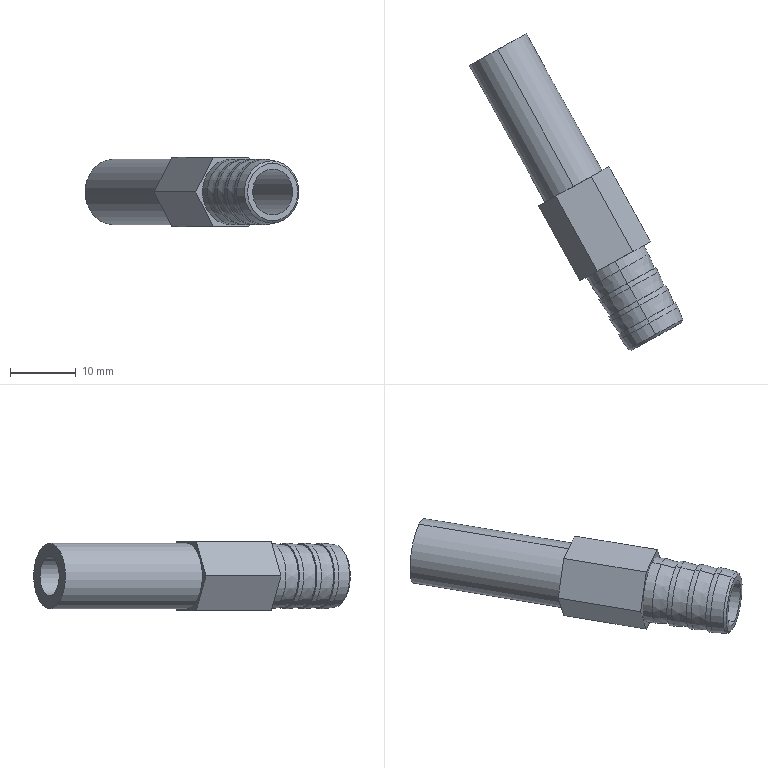Part | SolidWorks | features BaseBody 1 | 1 solid | 38 faces | box 32.611 x 48.276 x 10.659 mm | volume 2597 mm3 | cylinder 14 | plane 14 | cone 10 | commonest cylinder face diameters 10 x10 6 x2 7 x2
STEP:
#1=CARTESIAN_POINT('',(2.423,-77.341,-243.124));
#2=VERTEX_POINT('',#1);
#3=CARTESIAN_POINT('',(2.423,-77.341,-251.876));
#4=VERTEX_POINT('',#3);
#5=CARTESIAN_POINT('',(2.423,-77.341,-247.5));
#6=DIRECTION('',(-0.4848,0.8746,0.));
#7=DIRECTION('',(0.,0.,-1.));
#8=AXIS2_PLACEMENT_3D('',#5,#6,#7);
#9=CIRCLE('',#8,4.376);
#10=EDGE_CURVE('',#2,#4,#9,.T.);
#11=ORIENTED_EDGE('',*,*,#10,.T.);
#12=CARTESIAN_POINT('',(2.259,-77.045,-252.258));
#13=VERTEX_POINT('',#12);
#14=CARTESIAN_POINT('',(2.259,-77.045,-252.258));
#15=DIRECTION('',(-0.3212,0.5795,-0.749));
#16=VECTOR('',#15,1000.);
#17=LINE('',#14,#16);
#18=EDGE_CURVE('',#4,#13,#17,.T.);
#19=ORIENTED_EDGE('',*,*,#18,.T.);
#20=CARTESIAN_POINT('',(2.259,-77.045,-242.742));
#21=VERTEX_POINT('',#20);
#22=CARTESIAN_POINT('',(2.259,-77.045,-247.5));
#23=DIRECTION('',(0.4848,-0.8746,0.));
#24=DIRECTION('',(0.,0.,-1.));
#25=AXIS2_PLACEMENT_3D('',#22,#23,#24);
#26=CIRCLE('',#25,4.758);
#27=EDGE_CURVE('',#13,#21,#26,.T.);
#28=ORIENTED_EDGE('',*,*,#27,.T.);
#29=CARTESIAN_POINT('',(2.259,-77.045,-242.742));
#30=DIRECTION('',(-0.3212,0.5795,0.749));
#31=VECTOR('',#30,1000.);
#32=LINE('',#29,#31);
#33=EDGE_CURVE('',#2,#21,#32,.T.);
#34=ORIENTED_EDGE('',*,*,#33,.F.);
#35=EDGE_LOOP('',(#11,#19,#28,#34));
#36=FACE_OUTER_BOUND('',#35,.T.);
#37=CARTESIAN_POINT('',(2.259,-77.045,-247.5));
#38=DIRECTION('',(-0.4848,0.8746,0.));
#39=DIRECTION('',(0.,0.,1.));
#40=AXIS2_PLACEMENT_3D('',#37,#38,#39);
#41=CONICAL_SURFACE('',#40,4.758,0.8465);
#42=ADVANCED_FACE('',(#36),#41,.T.);
#43=CARTESIAN_POINT('',(-2.052,-69.267,-252.217));
#44=VERTEX_POINT('',#43);
#45=CARTESIAN_POINT('',(-2.052,-69.267,-242.783));
#46=VERTEX_POINT('',#45);
#47=CARTESIAN_POINT('',(-2.052,-69.267,-247.5));
#48=DIRECTION('',(0.4848,-0.8746,0.));
#49=DIRECTION('',(0.,0.,1.));
#50=AXIS2_PLACEMENT_3D('',#47,#48,#49);
#51=CIRCLE('',#50,4.717);
#52=EDGE_CURVE('',#44,#46,#51,.T.);
#53=ORIENTED_EDGE('',*,*,#52,.F.);
#54=CARTESIAN_POINT('',(-3.171,-67.249,-252.5));
#55=VERTEX_POINT('',#54);
#56=CARTESIAN_POINT('',(-3.171,-67.249,-252.5));
#57=DIRECTION('',(-0.4812,0.8681,-0.1219));
#58=VECTOR('',#57,1000.);
#59=LINE('',#56,#58);
#60=EDGE_CURVE('',#44,#55,#59,.T.);
#61=ORIENTED_EDGE('',*,*,#60,.T.);
#62=CARTESIAN_POINT('',(-3.171,-67.249,-242.5));
#63=VERTEX_POINT('',#62);
#64=CARTESIAN_POINT('',(-3.171,-67.249,-247.5));
#65=DIRECTION('',(0.4848,-0.8746,0.));
#66=DIRECTION('',(0.,0.,1.));
#67=AXIS2_PLACEMENT_3D('',#64,#65,#66);
#68=CIRCLE('',#67,5.);
#69=EDGE_CURVE('',#55,#63,#68,.T.);
#70=ORIENTED_EDGE('',*,*,#69,.T.);
#71=CARTESIAN_POINT('',(-3.171,-67.249,-242.5));
#72=DIRECTION('',(-0.4812,0.8681,0.1219));
#73=VECTOR('',#72,1000.);
#74=LINE('',#71,#73);
#75=EDGE_CURVE('',#46,#63,#74,.T.);
#76=ORIENTED_EDGE('',*,*,#75,.F.);
#77=EDGE_LOOP('',(#53,#61,#70,#76));
#78=FACE_OUTER_BOUND('',#77,.T.);
#79=CARTESIAN_POINT('',(-3.171,-67.249,-247.5));
#80=DIRECTION('',(-0.4848,0.8746,0.));
#81=DIRECTION('',(0.,0.,1.));
#82=AXIS2_PLACEMENT_3D('',#79,#80,#81);
#83=CONICAL_SURFACE('',#82,5.,0.1222);
#84=ADVANCED_FACE('',(#78),#83,.T.);
#85=CARTESIAN_POINT('',(-0.5605,-71.959,-252.217));
#86=VERTEX_POINT('',#85);
#87=CARTESIAN_POINT('',(-0.5605,-71.959,-242.783));
#88=VERTEX_POINT('',#87);
#89=CARTESIAN_POINT('',(-0.5605,-71.959,-247.5));
#90=DIRECTION('',(0.4848,-0.8746,0.));
#91=DIRECTION('',(0.,0.,1.));
#92=AXIS2_PLACEMENT_3D('',#89,#90,#91);
#93=CIRCLE('',#92,4.717);
#94=EDGE_CURVE('',#86,#88,#93,.T.);
#95=ORIENTED_EDGE('',*,*,#94,.F.);
#96=CARTESIAN_POINT('',(-1.679,-69.94,-252.5));
#97=VERTEX_POINT('',#96);
#98=CARTESIAN_POINT('',(-1.679,-69.94,-252.5));
#99=DIRECTION('',(-0.4812,0.8681,-0.1219));
#100=VECTOR('',#99,1000.);
#101=LINE('',#98,#100);
#102=EDGE_CURVE('',#86,#97,#101,.T.);
#103=ORIENTED_EDGE('',*,*,#102,.T.);
#104=CARTESIAN_POINT('',(-1.679,-69.94,-242.5));
#105=VERTEX_POINT('',#104);
#106=CARTESIAN_POINT('',(-1.679,-69.94,-247.5));
#107=DIRECTION('',(0.4848,-0.8746,0.));
#108=DIRECTION('',(0.,0.,1.));
#109=AXIS2_PLACEMENT_3D('',#106,#107,#108);
#110=CIRCLE('',#109,5.);
#111=EDGE_CURVE('',#97,#105,#110,.T.);
#112=ORIENTED_EDGE('',*,*,#111,.T.);
#113=CARTESIAN_POINT('',(-1.679,-69.94,-242.5));
#114=DIRECTION('',(-0.4812,0.8681,0.1219));
#115=VECTOR('',#114,1000.);
#116=LINE('',#113,#115);
#117=EDGE_CURVE('',#88,#105,#116,.T.);
#118=ORIENTED_EDGE('',*,*,#117,.F.);
#119=EDGE_LOOP('',(#95,#103,#112,#118));
#120=FACE_OUTER_BOUND('',#119,.T.);
#121=CARTESIAN_POINT('',(-1.679,-69.94,-247.5));
#122=DIRECTION('',(-0.4848,0.8746,0.));
#123=DIRECTION('',(0.,0.,1.));
#124=AXIS2_PLACEMENT_3D('',#121,#122,#123);
#125=CONICAL_SURFACE('',#124,5.,0.1222);
#126=ADVANCED_FACE('',(#120),#125,.T.);
#127=CARTESIAN_POINT('',(0.9313,-74.65,-252.217));
#128=VERTEX_POINT('',#127);
#129=CARTESIAN_POINT('',(0.9313,-74.65,-242.783));
#130=VERTEX_POINT('',#129);
#131=CARTESIAN_POINT('',(0.9313,-74.65,-247.5));
#132=DIRECTION('',(0.4848,-0.8746,0.));
#133=DIRECTION('',(0.,0.,1.));
#134=AXIS2_PLACEMENT_3D('',#131,#132,#133);
#135=CIRCLE('',#134,4.717);
#136=EDGE_CURVE('',#128,#130,#135,.T.);
#137=ORIENTED_EDGE('',*,*,#136,.F.);
#138=CARTESIAN_POINT('',(-0.1875,-72.631,-252.5));
#139=VERTEX_POINT('',#138);
#140=CARTESIAN_POINT('',(-0.1875,-72.631,-252.5));
#141=DIRECTION('',(-0.4812,0.8681,-0.1219));
#142=VECTOR('',#141,1000.);
#143=LINE('',#140,#142);
#144=EDGE_CURVE('',#128,#139,#143,.T.);
#145=ORIENTED_EDGE('',*,*,#144,.T.);
#146=CARTESIAN_POINT('',(-0.1875,-72.631,-242.5));
#147=VERTEX_POINT('',#146);
#148=CARTESIAN_POINT('',(-0.1875,-72.631,-247.5));
#149=DIRECTION('',(0.4848,-0.8746,0.));
#150=DIRECTION('',(0.,0.,1.));
#151=AXIS2_PLACEMENT_3D('',#148,#149,#150);
#152=CIRCLE('',#151,5.);
#153=EDGE_CURVE('',#139,#147,#152,.T.);
#154=ORIENTED_EDGE('',*,*,#153,.T.);
#155=CARTESIAN_POINT('',(-0.1875,-72.631,-242.5));
#156=DIRECTION('',(-0.4812,0.8681,0.1219));
#157=VECTOR('',#156,1000.);
#158=LINE('',#155,#157);
#159=EDGE_CURVE('',#130,#147,#158,.T.);
#160=ORIENTED_EDGE('',*,*,#159,.F.);
#161=EDGE_LOOP('',(#137,#145,#154,#160));
#162=FACE_OUTER_BOUND('',#161,.T.);
#163=CARTESIAN_POINT('',(-0.1875,-72.631,-247.5));
#164=DIRECTION('',(-0.4848,0.8746,0.));
#165=DIRECTION('',(0.,0.,1.));
#166=AXIS2_PLACEMENT_3D('',#163,#164,#165);
#167=CONICAL_SURFACE('',#166,5.,0.1222);
#168=ADVANCED_FACE('',(#162),#167,.T.);
#169=ORIENTED_EDGE('',*,*,#27,.F.);
#170=CARTESIAN_POINT('',(1.304,-75.322,-252.5));
#171=VERTEX_POINT('',#170);
#172=CARTESIAN_POINT('',(1.304,-75.322,-252.5));
#173=DIRECTION('',(-0.4812,0.8681,-0.1219));
#174=VECTOR('',#173,1000.);
#175=LINE('',#172,#174);
#176=EDGE_CURVE('',#13,#171,#175,.T.);
#177=ORIENTED_EDGE('',*,*,#176,.T.);
#178=CARTESIAN_POINT('',(1.304,-75.322,-242.5));
#179=VERTEX_POINT('',#178);
#180=CARTESIAN_POINT('',(1.304,-75.322,-247.5));
#181=DIRECTION('',(0.4848,-0.8746,0.));
#182=DIRECTION('',(0.,0.,1.));
#183=AXIS2_PLACEMENT_3D('',#180,#181,#182);
#184=CIRCLE('',#183,5.);
#185=EDGE_CURVE('',#171,#179,#184,.T.);
#186=ORIENTED_EDGE('',*,*,#185,.T.);
#187=CARTESIAN_POINT('',(1.304,-75.322,-242.5));
#188=DIRECTION('',(-0.4812,0.8681,0.1219));
#189=VECTOR('',#188,1000.);
#190=LINE('',#187,#189);
#191=EDGE_CURVE('',#21,#179,#190,.T.);
#192=ORIENTED_EDGE('',*,*,#191,.F.);
#193=EDGE_LOOP('',(#169,#177,#186,#192));
#194=FACE_OUTER_BOUND('',#193,.T.);
#195=CARTESIAN_POINT('',(1.304,-75.322,-247.5));
#196=DIRECTION('',(-0.4848,0.8746,0.));
#197=DIRECTION('',(0.,0.,1.));
#198=AXIS2_PLACEMENT_3D('',#195,#196,#197);
#199=CONICAL_SURFACE('',#198,5.,0.1222);
#200=ADVANCED_FACE('',(#194),#199,.T.);
#201=ORIENTED_EDGE('',*,*,#185,.F.);
#202=CARTESIAN_POINT('',(0.9313,-74.65,-252.5));
#203=VERTEX_POINT('',#202);
#204=CARTESIAN_POINT('',(2.423,-77.341,-252.5));
#205=DIRECTION('',(-0.4848,0.8746,0.));
#206=VECTOR('',#205,1000.);
#207=LINE('',#204,#206);
#208=EDGE_CURVE('',#171,#203,#207,.T.);
#209=ORIENTED_EDGE('',*,*,#208,.T.);
#210=CARTESIAN_POINT('',(0.9313,-74.65,-242.5));
#211=VERTEX_POINT('',#210);
#212=CARTESIAN_POINT('',(0.9313,-74.65,-247.5));
#213=DIRECTION('',(0.4848,-0.8746,0.));
#214=DIRECTION('',(0.,0.,1.));
#215=AXIS2_PLACEMENT_3D('',#212,#213,#214);
#216=CIRCLE('',#215,5.);
#217=EDGE_CURVE('',#203,#211,#216,.T.);
#218=ORIENTED_EDGE('',*,*,#217,.T.);
#219=CARTESIAN_POINT('',(2.423,-77.341,-242.5));
#220=DIRECTION('',(-0.4848,0.8746,0.));
#221=VECTOR('',#220,1000.);
#222=LINE('',#219,#221);
#223=EDGE_CURVE('',#179,#211,#222,.T.);
#224=ORIENTED_EDGE('',*,*,#223,.F.);
#225=EDGE_LOOP('',(#201,#209,#218,#224));
#226=FACE_OUTER_BOUND('',#225,.T.);
#227=CARTESIAN_POINT('',(2.423,-77.341,-247.5));
#228=DIRECTION('',(-0.4848,0.8746,0.));
#229=DIRECTION('',(0.,0.,1.));
#230=AXIS2_PLACEMENT_3D('',#227,#228,#229);
#231=CYLINDRICAL_SURFACE('',#230,5.);
#232=ADVANCED_FACE('',(#226),#231,.T.);
#233=ORIENTED_EDGE('',*,*,#153,.F.);
#234=CARTESIAN_POINT('',(-0.5605,-71.959,-252.5));
#235=VERTEX_POINT('',#234);
#236=CARTESIAN_POINT('',(2.423,-77.341,-252.5));
#237=DIRECTION('',(-0.4848,0.8746,0.));
#238=VECTOR('',#237,1000.);
#239=LINE('',#236,#238);
#240=EDGE_CURVE('',#139,#235,#239,.T.);
#241=ORIENTED_EDGE('',*,*,#240,.T.);
#242=CARTESIAN_POINT('',(-0.5605,-71.959,-242.5));
#243=VERTEX_POINT('',#242);
#244=CARTESIAN_POINT('',(-0.5605,-71.959,-247.5));
#245=DIRECTION('',(0.4848,-0.8746,0.));
#246=DIRECTION('',(0.,0.,1.));
#247=AXIS2_PLACEMENT_3D('',#244,#245,#246);
#248=CIRCLE('',#247,5.);
#249=EDGE_CURVE('',#235,#243,#248,.T.);
#250=ORIENTED_EDGE('',*,*,#249,.T.);
#251=CARTESIAN_POINT('',(2.423,-77.341,-242.5));
#252=DIRECTION('',(-0.4848,0.8746,0.));
#253=VECTOR('',#252,1000.);
#254=LINE('',#251,#253);
#255=EDGE_CURVE('',#147,#243,#254,.T.);
#256=ORIENTED_EDGE('',*,*,#255,.F.);
#257=EDGE_LOOP('',(#233,#241,#250,#256));
#258=FACE_OUTER_BOUND('',#257,.T.);
#259=CARTESIAN_POINT('',(2.423,-77.341,-247.5));
#260=DIRECTION('',(-0.4848,0.8746,0.));
#261=DIRECTION('',(0.,0.,1.));
#262=AXIS2_PLACEMENT_3D('',#259,#260,#261);
#263=CYLINDRICAL_SURFACE('',#262,5.);
#264=ADVANCED_FACE('',(#258),#263,.T.);
#265=ORIENTED_EDGE('',*,*,#111,.F.);
#266=CARTESIAN_POINT('',(-2.052,-69.267,-252.5));
#267=VERTEX_POINT('',#266);
#268=CARTESIAN_POINT('',(2.423,-77.341,-252.5));
#269=DIRECTION('',(-0.4848,0.8746,0.));
#270=VECTOR('',#269,1000.);
#271=LINE('',#268,#270);
#272=EDGE_CURVE('',#97,#267,#271,.T.);
#273=ORIENTED_EDGE('',*,*,#272,.T.);
#274=CARTESIAN_POINT('',(-2.052,-69.267,-242.5));
#275=VERTEX_POINT('',#274);
#276=CARTESIAN_POINT('',(-2.052,-69.267,-247.5));
#277=DIRECTION('',(0.4848,-0.8746,0.));
#278=DIRECTION('',(0.,0.,1.));
#279=AXIS2_PLACEMENT_3D('',#276,#277,#278);
#280=CIRCLE('',#279,5.);
#281=EDGE_CURVE('',#267,#275,#280,.T.);
#282=ORIENTED_EDGE('',*,*,#281,.T.);
#283=CARTESIAN_POINT('',(2.423,-77.341,-242.5));
#284=DIRECTION('',(-0.4848,0.8746,0.));
#285=VECTOR('',#284,1000.);
#286=LINE('',#283,#285);
#287=EDGE_CURVE('',#105,#275,#286,.T.);
#288=ORIENTED_EDGE('',*,*,#287,.F.);
#289=EDGE_LOOP('',(#265,#273,#282,#288));
#290=FACE_OUTER_BOUND('',#289,.T.);
#291=CARTESIAN_POINT('',(2.423,-77.341,-247.5));
#292=DIRECTION('',(-0.4848,0.8746,0.));
#293=DIRECTION('',(0.,0.,1.));
#294=AXIS2_PLACEMENT_3D('',#291,#292,#293);
#295=CYLINDRICAL_SURFACE('',#294,5.);
#296=ADVANCED_FACE('',(#290),#295,.T.);
#297=ORIENTED_EDGE('',*,*,#69,.F.);
#298=CARTESIAN_POINT('',(-3.917,-65.903,-252.5));
#299=VERTEX_POINT('',#298);
#300=CARTESIAN_POINT('',(-3.171,-67.249,-252.5));
#301=DIRECTION('',(-0.4848,0.8746,0.));
#302=VECTOR('',#301,1000.);
#303=LINE('',#300,#302);
#304=EDGE_CURVE('',#55,#299,#303,.T.);
#305=ORIENTED_EDGE('',*,*,#304,.T.);
#306=CARTESIAN_POINT('',(-3.917,-65.903,-242.5));
#307=VERTEX_POINT('',#306);
#308=CARTESIAN_POINT('',(-3.917,-65.903,-247.5));
#309=DIRECTION('',(0.4848,-0.8746,0.));
#310=DIRECTION('',(0.,0.,-1.));
#311=AXIS2_PLACEMENT_3D('',#308,#309,#310);
#312=CIRCLE('',#311,5.);
#313=EDGE_CURVE('',#299,#307,#312,.T.);
#314=ORIENTED_EDGE('',*,*,#313,.T.);
#315=CARTESIAN_POINT('',(-3.171,-67.249,-242.5));
#316=DIRECTION('',(-0.4848,0.8746,0.));
#317=VECTOR('',#316,1000.);
#318=LINE('',#315,#317);
#319=EDGE_CURVE('',#63,#307,#318,.T.);
#320=ORIENTED_EDGE('',*,*,#319,.F.);
#321=EDGE_LOOP('',(#297,#305,#314,#320));
#322=FACE_OUTER_BOUND('',#321,.T.);
#323=CARTESIAN_POINT('',(-3.171,-67.249,-247.5));
#324=DIRECTION('',(-0.4848,0.8746,0.));
#325=DIRECTION('',(0.,0.,1.));
#326=AXIS2_PLACEMENT_3D('',#323,#324,#325);
#327=CYLINDRICAL_SURFACE('',#326,5.);
#328=ADVANCED_FACE('',(#322),#327,.T.);
#329=CARTESIAN_POINT('',(-3.917,-65.903,-244.));
#330=VERTEX_POINT('',#329);
#331=CARTESIAN_POINT('',(-3.917,-65.903,-251.));
#332=VERTEX_POINT('',#331);
#333=CARTESIAN_POINT('',(-3.917,-65.903,-247.5));
#334=DIRECTION('',(0.4848,-0.8746,0.));
#335=DIRECTION('',(0.,0.,-1.));
#336=AXIS2_PLACEMENT_3D('',#333,#334,#335);
#337=CIRCLE('',#336,3.5);
#338=EDGE_CURVE('',#330,#332,#337,.T.);
#339=ORIENTED_EDGE('',*,*,#338,.F.);
#340=CARTESIAN_POINT('',(2.423,-77.341,-244.));
#341=VERTEX_POINT('',#340);
#342=CARTESIAN_POINT('',(-21.818,-33.61,-244.));
#343=DIRECTION('',(0.4848,-0.8746,0.));
#344=VECTOR('',#343,1000.);
#345=LINE('',#342,#344);
#346=EDGE_CURVE('',#330,#341,#345,.T.);
#347=ORIENTED_EDGE('',*,*,#346,.T.);
#348=CARTESIAN_POINT('',(2.423,-77.341,-251.));
#349=VERTEX_POINT('',#348);
#350=CARTESIAN_POINT('',(2.423,-77.341,-247.5));
#351=DIRECTION('',(-0.4848,0.8746,0.));
#352=DIRECTION('',(-0.586,-0.3248,0.7423));
#353=AXIS2_PLACEMENT_3D('',#350,#351,#352);
#354=CIRCLE('',#353,3.5);
#355=EDGE_CURVE('',#349,#341,#354,.T.);
#356=ORIENTED_EDGE('',*,*,#355,.F.);
#357=CARTESIAN_POINT('',(-21.818,-33.61,-251.));
#358=DIRECTION('',(0.4848,-0.8746,0.));
#359=VECTOR('',#358,1000.);
#360=LINE('',#357,#359);
#361=EDGE_CURVE('',#332,#349,#360,.T.);
#362=ORIENTED_EDGE('',*,*,#361,.F.);
#363=EDGE_LOOP('',(#339,#347,#356,#362));
#364=FACE_OUTER_BOUND('',#363,.T.);
#365=CARTESIAN_POINT('',(-21.818,-33.61,-247.5));
#366=DIRECTION('',(0.4848,-0.8746,0.));
#367=DIRECTION('',(0.,0.,-1.));
#368=AXIS2_PLACEMENT_3D('',#365,#366,#367);
#369=CYLINDRICAL_SURFACE('',#368,3.5);
#370=ADVANCED_FACE('',(#364),#369,.F.);
#371=CARTESIAN_POINT('',(-10.257,-54.466,-252.5));
#372=VERTEX_POINT('',#371);
#373=CARTESIAN_POINT('',(-10.257,-54.466,-242.5));
#374=VERTEX_POINT('',#373);
#375=CARTESIAN_POINT('',(-10.257,-54.466,-247.5));
#376=DIRECTION('',(0.4848,-0.8746,0.));
#377=DIRECTION('',(0.,0.,-1.));
#378=AXIS2_PLACEMENT_3D('',#375,#376,#377);
#379=CIRCLE('',#378,5.);
#380=EDGE_CURVE('',#372,#374,#379,.T.);
#381=ORIENTED_EDGE('',*,*,#380,.F.);
#382=CARTESIAN_POINT('',(-21.817,-33.611,-252.5));
#383=VERTEX_POINT('',#382);
#384=CARTESIAN_POINT('',(-60.602,36.359,-252.5));
#385=DIRECTION('',(-0.4848,0.8746,0.));
#386=VECTOR('',#385,1000.);
#387=LINE('',#384,#386);
#388=EDGE_CURVE('',#372,#383,#387,.T.);
#389=ORIENTED_EDGE('',*,*,#388,.T.);
#390=CARTESIAN_POINT('',(-21.817,-33.611,-242.5));
#391=VERTEX_POINT('',#390);
#392=CARTESIAN_POINT('',(-21.817,-33.611,-247.5));
#393=DIRECTION('',(0.4848,-0.8746,0.));
#394=DIRECTION('',(0.,0.,1.));
#395=AXIS2_PLACEMENT_3D('',#392,#393,#394);
#396=CIRCLE('',#395,5.);
#397=EDGE_CURVE('',#383,#391,#396,.T.);
#398=ORIENTED_EDGE('',*,*,#397,.T.);
#399=CARTESIAN_POINT('',(-60.602,36.359,-242.5));
#400=DIRECTION('',(-0.4848,0.8746,0.));
#401=VECTOR('',#400,1000.);
#402=LINE('',#399,#401);
#403=EDGE_CURVE('',#374,#391,#402,.T.);
#404=ORIENTED_EDGE('',*,*,#403,.F.);
#405=EDGE_LOOP('',(#381,#389,#398,#404));
#406=FACE_OUTER_BOUND('',#405,.T.);
#407=CARTESIAN_POINT('',(-60.602,36.359,-247.5));
#408=DIRECTION('',(-0.4848,0.8746,0.));
#409=DIRECTION('',(0.,0.,1.));
#410=AXIS2_PLACEMENT_3D('',#407,#408,#409);
#411=CYLINDRICAL_SURFACE('',#410,5.);
#412=ADVANCED_FACE('',(#406),#411,.T.);
#413=CARTESIAN_POINT('',(-3.917,-65.903,-244.5));
#414=VERTEX_POINT('',#413);
#415=CARTESIAN_POINT('',(-3.917,-65.903,-250.5));
#416=VERTEX_POINT('',#415);
#417=CARTESIAN_POINT('',(-3.917,-65.903,-247.5));
#418=DIRECTION('',(0.4848,-0.8746,0.));
#419=DIRECTION('',(0.,0.,-1.));
#420=AXIS2_PLACEMENT_3D('',#417,#418,#419);
#421=CIRCLE('',#420,3.);
#422=EDGE_CURVE('',#414,#416,#421,.T.);
#423=ORIENTED_EDGE('',*,*,#422,.T.);
#424=CARTESIAN_POINT('',(-21.817,-33.611,-250.5));
#425=VERTEX_POINT('',#424);
#426=CARTESIAN_POINT('',(-5.818,-62.473,-250.5));
#427=DIRECTION('',(-0.4848,0.8746,0.));
#428=VECTOR('',#427,1000.);
#429=LINE('',#426,#428);
#430=EDGE_CURVE('',#416,#425,#429,.T.);
#431=ORIENTED_EDGE('',*,*,#430,.T.);
#432=CARTESIAN_POINT('',(-21.817,-33.611,-244.5));
#433=VERTEX_POINT('',#432);
#434=CARTESIAN_POINT('',(-21.817,-33.611,-247.5));
#435=DIRECTION('',(-0.4848,0.8746,0.));
#436=DIRECTION('',(0.,0.,1.));
#437=AXIS2_PLACEMENT_3D('',#434,#435,#436);
#438=CIRCLE('',#437,3.);
#439=EDGE_CURVE('',#425,#433,#438,.T.);
#440=ORIENTED_EDGE('',*,*,#439,.T.);
#441=CARTESIAN_POINT('',(-5.818,-62.473,-244.5));
#442=DIRECTION('',(-0.4848,0.8746,0.));
#443=VECTOR('',#442,1000.);
#444=LINE('',#441,#443);
#445=EDGE_CURVE('',#414,#433,#444,.T.);
#446=ORIENTED_EDGE('',*,*,#445,.F.);
#447=EDGE_LOOP('',(#423,#431,#440,#446));
#448=FACE_OUTER_BOUND('',#447,.T.);
#449=CARTESIAN_POINT('',(-5.818,-62.473,-247.5));
#450=DIRECTION('',(-0.4848,0.8746,0.));
#451=DIRECTION('',(0.,0.,1.));
#452=AXIS2_PLACEMENT_3D('',#449,#450,#451);
#453=CYLINDRICAL_SURFACE('',#452,3.);
#454=ADVANCED_FACE('',(#448),#453,.F.);
#455=ORIENTED_EDGE('',*,*,#430,.F.);
#456=CARTESIAN_POINT('',(-3.917,-65.903,-247.5));
#457=DIRECTION('',(0.4848,-0.8746,0.));
#458=DIRECTION('',(0.,0.,-1.));
#459=AXIS2_PLACEMENT_3D('',#456,#457,#458);
#460=CIRCLE('',#459,3.);
#461=EDGE_CURVE('',#416,#414,#460,.T.);
#462=ORIENTED_EDGE('',*,*,#461,.T.);
#463=ORIENTED_EDGE('',*,*,#445,.T.);
#464=CARTESIAN_POINT('',(-21.817,-33.611,-247.5));
#465=DIRECTION('',(-0.4848,0.8746,0.));
#466=DIRECTION('',(0.,0.,1.));
#467=AXIS2_PLACEMENT_3D('',#464,#465,#466);
#468=CIRCLE('',#467,3.);
#469=EDGE_CURVE('',#433,#425,#468,.T.);
#470=ORIENTED_EDGE('',*,*,#469,.T.);
#471=EDGE_LOOP('',(#455,#462,#463,#470));
#472=FACE_OUTER_BOUND('',#471,.T.);
#473=CARTESIAN_POINT('',(-5.818,-62.473,-247.5));
#474=DIRECTION('',(-0.4848,0.8746,0.));
#475=DIRECTION('',(0.,0.,1.));
#476=AXIS2_PLACEMENT_3D('',#473,#474,#475);
#477=CYLINDRICAL_SURFACE('',#476,3.);
#478=ADVANCED_FACE('',(#472),#477,.F.);
#479=ORIENTED_EDGE('',*,*,#388,.F.);
#480=CARTESIAN_POINT('',(-10.257,-54.466,-247.5));
#481=DIRECTION('',(0.4848,-0.8746,0.));
#482=DIRECTION('',(0.,0.,-1.));
#483=AXIS2_PLACEMENT_3D('',#480,#481,#482);
#484=CIRCLE('',#483,5.);
#485=EDGE_CURVE('',#374,#372,#484,.T.);
#486=ORIENTED_EDGE('',*,*,#485,.F.);
#487=ORIENTED_EDGE('',*,*,#403,.T.);
#488=CARTESIAN_POINT('',(-21.817,-33.611,-247.5));
#489=DIRECTION('',(0.4848,-0.8746,0.));
#490=DIRECTION('',(0.,0.,1.));
#491=AXIS2_PLACEMENT_3D('',#488,#489,#490);
#492=CIRCLE('',#491,5.);
#493=EDGE_CURVE('',#391,#383,#492,.T.);
#494=ORIENTED_EDGE('',*,*,#493,.T.);
#495=EDGE_LOOP('',(#479,#486,#487,#494));
#496=FACE_OUTER_BOUND('',#495,.T.);
#497=CARTESIAN_POINT('',(-60.602,36.359,-247.5));
#498=DIRECTION('',(-0.4848,0.8746,0.));
#499=DIRECTION('',(0.,0.,1.));
#500=AXIS2_PLACEMENT_3D('',#497,#498,#499);
#501=CYLINDRICAL_SURFACE('',#500,5.);
#502=ADVANCED_FACE('',(#496),#501,.T.);
#503=CARTESIAN_POINT('',(-3.917,-65.903,-247.5));
#504=DIRECTION('',(0.4848,-0.8746,0.));
#505=DIRECTION('',(0.,0.,-1.));
#506=AXIS2_PLACEMENT_3D('',#503,#504,#505);
#507=CIRCLE('',#506,3.5);
#508=EDGE_CURVE('',#332,#330,#507,.T.);
#509=ORIENTED_EDGE('',*,*,#508,.T.);
#510=ORIENTED_EDGE('',*,*,#338,.T.);
#511=EDGE_LOOP('',(#509,#510));
#512=FACE_OUTER_BOUND('',#511,.T.);
#513=ORIENTED_EDGE('',*,*,#422,.F.);
#514=ORIENTED_EDGE('',*,*,#461,.F.);
#515=EDGE_LOOP('',(#513,#514));
#516=FACE_BOUND('',#515,.T.);
#517=CARTESIAN_POINT('',(-3.917,-65.903,-247.5));
#518=DIRECTION('',(0.4848,-0.8746,0.));
#519=DIRECTION('',(0.,0.,1.));
#520=AXIS2_PLACEMENT_3D('',#517,#518,#519);
#521=PLANE('',#520);
#522=ADVANCED_FACE('',(#512,#516),#521,.T.);
#523=ORIENTED_EDGE('',*,*,#346,.F.);
#524=ORIENTED_EDGE('',*,*,#508,.F.);
#525=ORIENTED_EDGE('',*,*,#361,.T.);
#526=CARTESIAN_POINT('',(2.423,-77.341,-247.5));
#527=DIRECTION('',(-0.4848,0.8746,0.));
#528=DIRECTION('',(-0.586,-0.3248,0.7423));
#529=AXIS2_PLACEMENT_3D('',#526,#527,#528);
#530=CIRCLE('',#529,3.5);
#531=EDGE_CURVE('',#341,#349,#530,.T.);
#532=ORIENTED_EDGE('',*,*,#531,.F.);
#533=EDGE_LOOP('',(#523,#524,#525,#532));
#534=FACE_OUTER_BOUND('',#533,.T.);
#535=CARTESIAN_POINT('',(-21.818,-33.61,-247.5));
#536=DIRECTION('',(0.4848,-0.8746,0.));
#537=DIRECTION('',(0.,0.,-1.));
#538=AXIS2_PLACEMENT_3D('',#535,#536,#537);
#539=CYLINDRICAL_SURFACE('',#538,3.5);
#540=ADVANCED_FACE('',(#534),#539,.F.);
#541=CARTESIAN_POINT('',(-4.874,-51.483,-247.5));
#542=VERTEX_POINT('',#541);
#543=CARTESIAN_POINT('',(-7.566,-52.974,-242.171));
#544=VERTEX_POINT('',#543);
#545=CARTESIAN_POINT('',(-4.874,-51.483,-247.5));
#546=DIRECTION('',(-0.4373,-0.2424,0.866));
#547=VECTOR('',#546,1000.);
#548=LINE('',#545,#547);
#549=EDGE_CURVE('',#542,#544,#548,.T.);
#550=ORIENTED_EDGE('',*,*,#549,.F.);
#551=CARTESIAN_POINT('',(-7.566,-52.974,-252.829));
#552=VERTEX_POINT('',#551);
#553=CARTESIAN_POINT('',(-7.566,-52.974,-252.829));
#554=DIRECTION('',(0.4373,0.2424,0.866));
#555=VECTOR('',#554,1000.);
#556=LINE('',#553,#555);
#557=EDGE_CURVE('',#552,#542,#556,.T.);
#558=ORIENTED_EDGE('',*,*,#557,.F.);
#559=CARTESIAN_POINT('',(-12.948,-55.958,-252.829));
#560=VERTEX_POINT('',#559);
#561=CARTESIAN_POINT('',(-12.948,-55.958,-252.829));
#562=DIRECTION('',(0.8746,0.4848,0.));
#563=VECTOR('',#562,1000.);
#564=LINE('',#561,#563);
#565=EDGE_CURVE('',#560,#552,#564,.T.);
#566=ORIENTED_EDGE('',*,*,#565,.F.);
#567=CARTESIAN_POINT('',(-15.639,-57.45,-247.5));
#568=VERTEX_POINT('',#567);
#569=CARTESIAN_POINT('',(-15.639,-57.45,-247.5));
#570=DIRECTION('',(0.4373,0.2424,-0.866));
#571=VECTOR('',#570,1000.);
#572=LINE('',#569,#571);
#573=EDGE_CURVE('',#568,#560,#572,.T.);
#574=ORIENTED_EDGE('',*,*,#573,.F.);
#575=CARTESIAN_POINT('',(-12.948,-55.958,-242.171));
#576=VERTEX_POINT('',#575);
#577=CARTESIAN_POINT('',(-12.948,-55.958,-242.171));
#578=DIRECTION('',(-0.4373,-0.2424,-0.866));
#579=VECTOR('',#578,1000.);
#580=LINE('',#577,#579);
#581=EDGE_CURVE('',#576,#568,#580,.T.);
#582=ORIENTED_EDGE('',*,*,#581,.F.);
#583=CARTESIAN_POINT('',(-7.566,-52.974,-242.171));
#584=DIRECTION('',(-0.8746,-0.4848,0.));
#585=VECTOR('',#584,1000.);
#586=LINE('',#583,#585);
#587=EDGE_CURVE('',#544,#576,#586,.T.);
#588=ORIENTED_EDGE('',*,*,#587,.F.);
#589=EDGE_LOOP('',(#550,#558,#566,#574,#582,#588));
#590=FACE_OUTER_BOUND('',#589,.T.);
#591=ORIENTED_EDGE('',*,*,#485,.T.);
#592=ORIENTED_EDGE('',*,*,#380,.T.);
#593=EDGE_LOOP('',(#591,#592));
#594=FACE_BOUND('',#593,.T.);
#595=CARTESIAN_POINT('',(-10.257,-54.466,-247.5));
#596=DIRECTION('',(0.4848,-0.8746,0.));
#597=DIRECTION('',(0.,0.,1.));
#598=AXIS2_PLACEMENT_3D('',#595,#596,#597);
#599=PLANE('',#598);
#600=ADVANCED_FACE('',(#590,#594),#599,.F.);
#601=CARTESIAN_POINT('',(-1.226,-64.412,-252.829));
#602=VERTEX_POINT('',#601);
#603=CARTESIAN_POINT('',(1.465,-62.92,-247.5));
#604=VERTEX_POINT('',#603);
#605=CARTESIAN_POINT('',(-1.226,-64.412,-252.829));
#606=DIRECTION('',(0.4373,0.2424,0.866));
#607=VECTOR('',#606,1000.);
#608=LINE('',#605,#607);
#609=EDGE_CURVE('',#602,#604,#608,.T.);
#610=ORIENTED_EDGE('',*,*,#609,.F.);
#611=CARTESIAN_POINT('',(-9.803,-48.938,-252.829));
#612=DIRECTION('',(0.4848,-0.8746,0.));
#613=VECTOR('',#612,1000.);
#614=LINE('',#611,#613);
#615=EDGE_CURVE('',#552,#602,#614,.T.);
#616=ORIENTED_EDGE('',*,*,#615,.F.);
#617=ORIENTED_EDGE('',*,*,#557,.T.);
#618=CARTESIAN_POINT('',(-7.112,-47.446,-247.5));
#619=DIRECTION('',(0.4848,-0.8746,0.));
#620=VECTOR('',#619,1000.);
#621=LINE('',#618,#620);
#622=EDGE_CURVE('',#542,#604,#621,.T.);
#623=ORIENTED_EDGE('',*,*,#622,.T.);
#624=EDGE_LOOP('',(#610,#616,#617,#623));
#625=FACE_OUTER_BOUND('',#624,.T.);
#626=CARTESIAN_POINT('',(-9.803,-48.938,-252.829));
#627=DIRECTION('',(0.7574,0.4199,-0.5));
#628=DIRECTION('',(0.4373,0.2424,0.866));
#629=AXIS2_PLACEMENT_3D('',#626,#627,#628);
#630=PLANE('',#629);
#631=ADVANCED_FACE('',(#625),#630,.T.);
#632=CARTESIAN_POINT('',(-6.608,-67.395,-252.829));
#633=VERTEX_POINT('',#632);
#634=CARTESIAN_POINT('',(-6.608,-67.395,-252.829));
#635=DIRECTION('',(0.8746,0.4848,0.));
#636=VECTOR('',#635,1000.);
#637=LINE('',#634,#636);
#638=EDGE_CURVE('',#633,#602,#637,.T.);
#639=ORIENTED_EDGE('',*,*,#638,.F.);
#640=CARTESIAN_POINT('',(-15.185,-51.921,-252.829));
#641=DIRECTION('',(0.4848,-0.8746,0.));
#642=VECTOR('',#641,1000.);
#643=LINE('',#640,#642);
#644=EDGE_CURVE('',#560,#633,#643,.T.);
#645=ORIENTED_EDGE('',*,*,#644,.F.);
#646=ORIENTED_EDGE('',*,*,#565,.T.);
#647=ORIENTED_EDGE('',*,*,#615,.T.);
#648=EDGE_LOOP('',(#639,#645,#646,#647));
#649=FACE_OUTER_BOUND('',#648,.T.);
#650=CARTESIAN_POINT('',(-15.185,-51.921,-252.829));
#651=DIRECTION('',(0.,0.,-1.));
#652=DIRECTION('',(0.8746,0.4848,0.));
#653=AXIS2_PLACEMENT_3D('',#650,#651,#652);
#654=PLANE('',#653);
#655=ADVANCED_FACE('',(#649),#654,.T.);
#656=CARTESIAN_POINT('',(-9.299,-68.887,-247.5));
#657=VERTEX_POINT('',#656);
#658=CARTESIAN_POINT('',(-9.299,-68.887,-247.5));
#659=DIRECTION('',(0.4373,0.2424,-0.866));
#660=VECTOR('',#659,1000.);
#661=LINE('',#658,#660);
#662=EDGE_CURVE('',#657,#633,#661,.T.);
#663=ORIENTED_EDGE('',*,*,#662,.F.);
#664=CARTESIAN_POINT('',(-17.877,-53.413,-247.5));
#665=DIRECTION('',(0.4848,-0.8746,0.));
#666=VECTOR('',#665,1000.);
#667=LINE('',#664,#666);
#668=EDGE_CURVE('',#568,#657,#667,.T.);
#669=ORIENTED_EDGE('',*,*,#668,.F.);
#670=ORIENTED_EDGE('',*,*,#573,.T.);
#671=ORIENTED_EDGE('',*,*,#644,.T.);
#672=EDGE_LOOP('',(#663,#669,#670,#671));
#673=FACE_OUTER_BOUND('',#672,.T.);
#674=CARTESIAN_POINT('',(-17.877,-53.413,-247.5));
#675=DIRECTION('',(-0.7574,-0.4199,-0.5));
#676=DIRECTION('',(0.4373,0.2424,-0.866));
#677=AXIS2_PLACEMENT_3D('',#674,#675,#676);
#678=PLANE('',#677);
#679=ADVANCED_FACE('',(#673),#678,.T.);
#680=CARTESIAN_POINT('',(-6.608,-67.395,-242.171));
#681=VERTEX_POINT('',#680);
#682=CARTESIAN_POINT('',(-6.608,-67.395,-242.171));
#683=DIRECTION('',(-0.4373,-0.2424,-0.866));
#684=VECTOR('',#683,1000.);
#685=LINE('',#682,#684);
#686=EDGE_CURVE('',#681,#657,#685,.T.);
#687=ORIENTED_EDGE('',*,*,#686,.F.);
#688=CARTESIAN_POINT('',(-15.185,-51.921,-242.171));
#689=DIRECTION('',(0.4848,-0.8746,0.));
#690=VECTOR('',#689,1000.);
#691=LINE('',#688,#690);
#692=EDGE_CURVE('',#576,#681,#691,.T.);
#693=ORIENTED_EDGE('',*,*,#692,.F.);
#694=ORIENTED_EDGE('',*,*,#581,.T.);
#695=ORIENTED_EDGE('',*,*,#668,.T.);
#696=EDGE_LOOP('',(#687,#693,#694,#695));
#697=FACE_OUTER_BOUND('',#696,.T.);
#698=CARTESIAN_POINT('',(-15.185,-51.921,-242.171));
#699=DIRECTION('',(-0.7574,-0.4199,0.5));
#700=DIRECTION('',(-0.4373,-0.2424,-0.866));
#701=AXIS2_PLACEMENT_3D('',#698,#699,#700);
#702=PLANE('',#701);
#703=ADVANCED_FACE('',(#697),#702,.T.);
#704=CARTESIAN_POINT('',(-1.226,-64.412,-242.171));
#705=VERTEX_POINT('',#704);
#706=CARTESIAN_POINT('',(-1.226,-64.412,-242.171));
#707=DIRECTION('',(-0.8746,-0.4848,0.));
#708=VECTOR('',#707,1000.);
#709=LINE('',#706,#708);
#710=EDGE_CURVE('',#705,#681,#709,.T.);
#711=ORIENTED_EDGE('',*,*,#710,.F.);
#712=CARTESIAN_POINT('',(-9.803,-48.938,-242.171));
#713=DIRECTION('',(0.4848,-0.8746,0.));
#714=VECTOR('',#713,1000.);
#715=LINE('',#712,#714);
#716=EDGE_CURVE('',#544,#705,#715,.T.);
#717=ORIENTED_EDGE('',*,*,#716,.F.);
#718=ORIENTED_EDGE('',*,*,#587,.T.);
#719=ORIENTED_EDGE('',*,*,#692,.T.);
#720=EDGE_LOOP('',(#711,#717,#718,#719));
#721=FACE_OUTER_BOUND('',#720,.T.);
#722=CARTESIAN_POINT('',(-9.803,-48.938,-242.171));
#723=DIRECTION('',(0.,0.,1.));
#724=DIRECTION('',(-0.8746,-0.4848,0.));
#725=AXIS2_PLACEMENT_3D('',#722,#723,#724);
#726=PLANE('',#725);
#727=ADVANCED_FACE('',(#721),#726,.T.);
#728=ORIENTED_EDGE('',*,*,#622,.F.);
#729=ORIENTED_EDGE('',*,*,#549,.T.);
#730=ORIENTED_EDGE('',*,*,#716,.T.);
#731=CARTESIAN_POINT('',(1.465,-62.92,-247.5));
#732=DIRECTION('',(-0.4373,-0.2424,0.866));
#733=VECTOR('',#732,1000.);
#734=LINE('',#731,#733);
#735=EDGE_CURVE('',#604,#705,#734,.T.);
#736=ORIENTED_EDGE('',*,*,#735,.F.);
#737=EDGE_LOOP('',(#728,#729,#730,#736));
#738=FACE_OUTER_BOUND('',#737,.T.);
#739=CARTESIAN_POINT('',(-7.112,-47.446,-247.5));
#740=DIRECTION('',(0.7574,0.4199,0.5));
#741=DIRECTION('',(-0.4373,-0.2424,0.866));
#742=AXIS2_PLACEMENT_3D('',#739,#740,#741);
#743=PLANE('',#742);
#744=ADVANCED_FACE('',(#738),#743,.T.);
#745=ORIENTED_EDGE('',*,*,#304,.F.);
#746=CARTESIAN_POINT('',(-3.171,-67.249,-247.5));
#747=DIRECTION('',(0.4848,-0.8746,0.));
#748=DIRECTION('',(0.,0.,1.));
#749=AXIS2_PLACEMENT_3D('',#746,#747,#748);
#750=CIRCLE('',#749,5.);
#751=EDGE_CURVE('',#63,#55,#750,.T.);
#752=ORIENTED_EDGE('',*,*,#751,.F.);
#753=ORIENTED_EDGE('',*,*,#319,.T.);
#754=CARTESIAN_POINT('',(-3.917,-65.903,-247.5));
#755=DIRECTION('',(0.4848,-0.8746,0.));
#756=DIRECTION('',(0.,0.,-1.));
#757=AXIS2_PLACEMENT_3D('',#754,#755,#756);
#758=CIRCLE('',#757,5.);
#759=EDGE_CURVE('',#307,#299,#758,.T.);
#760=ORIENTED_EDGE('',*,*,#759,.T.);
#761=EDGE_LOOP('',(#745,#752,#753,#760));
#762=FACE_OUTER_BOUND('',#761,.T.);
#763=CARTESIAN_POINT('',(-3.171,-67.249,-247.5));
#764=DIRECTION('',(-0.4848,0.8746,0.));
#765=DIRECTION('',(0.,0.,1.));
#766=AXIS2_PLACEMENT_3D('',#763,#764,#765);
#767=CYLINDRICAL_SURFACE('',#766,5.);
#768=ADVANCED_FACE('',(#762),#767,.T.);
#769=ORIENTED_EDGE('',*,*,#272,.F.);
#770=CARTESIAN_POINT('',(-1.679,-69.94,-247.5));
#771=DIRECTION('',(0.4848,-0.8746,0.));
#772=DIRECTION('',(0.,0.,1.));
#773=AXIS2_PLACEMENT_3D('',#770,#771,#772);
#774=CIRCLE('',#773,5.);
#775=EDGE_CURVE('',#105,#97,#774,.T.);
#776=ORIENTED_EDGE('',*,*,#775,.F.);
#777=ORIENTED_EDGE('',*,*,#287,.T.);
#778=CARTESIAN_POINT('',(-2.052,-69.267,-247.5));
#779=DIRECTION('',(0.4848,-0.8746,0.));
#780=DIRECTION('',(0.,0.,1.));
#781=AXIS2_PLACEMENT_3D('',#778,#779,#780);
#782=CIRCLE('',#781,5.);
#783=EDGE_CURVE('',#275,#267,#782,.T.);
#784=ORIENTED_EDGE('',*,*,#783,.T.);
#785=EDGE_LOOP('',(#769,#776,#777,#784));
#786=FACE_OUTER_BOUND('',#785,.T.);
#787=CARTESIAN_POINT('',(2.423,-77.341,-247.5));
#788=DIRECTION('',(-0.4848,0.8746,0.));
#789=DIRECTION('',(0.,0.,1.));
#790=AXIS2_PLACEMENT_3D('',#787,#788,#789);
#791=CYLINDRICAL_SURFACE('',#790,5.);
#792=ADVANCED_FACE('',(#786),#791,.T.);
#793=ORIENTED_EDGE('',*,*,#240,.F.);
#794=CARTESIAN_POINT('',(-0.1875,-72.631,-247.5));
#795=DIRECTION('',(0.4848,-0.8746,0.));
#796=DIRECTION('',(0.,0.,1.));
#797=AXIS2_PLACEMENT_3D('',#794,#795,#796);
#798=CIRCLE('',#797,5.);
#799=EDGE_CURVE('',#147,#139,#798,.T.);
#800=ORIENTED_EDGE('',*,*,#799,.F.);
#801=ORIENTED_EDGE('',*,*,#255,.T.);
#802=CARTESIAN_POINT('',(-0.5605,-71.959,-247.5));
#803=DIRECTION('',(0.4848,-0.8746,0.));
#804=DIRECTION('',(0.,0.,1.));
#805=AXIS2_PLACEMENT_3D('',#802,#803,#804);
#806=CIRCLE('',#805,5.);
#807=EDGE_CURVE('',#243,#235,#806,.T.);
#808=ORIENTED_EDGE('',*,*,#807,.T.);
#809=EDGE_LOOP('',(#793,#800,#801,#808));
#810=FACE_OUTER_BOUND('',#809,.T.);
#811=CARTESIAN_POINT('',(2.423,-77.341,-247.5));
#812=DIRECTION('',(-0.4848,0.8746,0.));
#813=DIRECTION('',(0.,0.,1.));
#814=AXIS2_PLACEMENT_3D('',#811,#812,#813);
#815=CYLINDRICAL_SURFACE('',#814,5.);
#816=ADVANCED_FACE('',(#810),#815,.T.);
#817=ORIENTED_EDGE('',*,*,#208,.F.);
#818=CARTESIAN_POINT('',(1.304,-75.322,-247.5));
#819=DIRECTION('',(0.4848,-0.8746,0.));
#820=DIRECTION('',(0.,0.,1.));
#821=AXIS2_PLACEMENT_3D('',#818,#819,#820);
#822=CIRCLE('',#821,5.);
#823=EDGE_CURVE('',#179,#171,#822,.T.);
#824=ORIENTED_EDGE('',*,*,#823,.F.);
#825=ORIENTED_EDGE('',*,*,#223,.T.);
#826=CARTESIAN_POINT('',(0.9313,-74.65,-247.5));
#827=DIRECTION('',(0.4848,-0.8746,0.));
#828=DIRECTION('',(0.,0.,1.));
#829=AXIS2_PLACEMENT_3D('',#826,#827,#828);
#830=CIRCLE('',#829,5.);
#831=EDGE_CURVE('',#211,#203,#830,.T.);
#832=ORIENTED_EDGE('',*,*,#831,.T.);
#833=EDGE_LOOP('',(#817,#824,#825,#832));
#834=FACE_OUTER_BOUND('',#833,.T.);
#835=CARTESIAN_POINT('',(2.423,-77.341,-247.5));
#836=DIRECTION('',(-0.4848,0.8746,0.));
#837=DIRECTION('',(0.,0.,1.));
#838=AXIS2_PLACEMENT_3D('',#835,#836,#837);
#839=CYLINDRICAL_SURFACE('',#838,5.);
#840=ADVANCED_FACE('',(#834),#839,.T.);
#841=ORIENTED_EDGE('',*,*,#355,.T.);
#842=ORIENTED_EDGE('',*,*,#531,.T.);
#843=EDGE_LOOP('',(#841,#842));
#844=FACE_BOUND('',#843,.T.);
#845=ORIENTED_EDGE('',*,*,#10,.F.);
#846=CARTESIAN_POINT('',(2.423,-77.341,-247.5));
#847=DIRECTION('',(-0.4848,0.8746,0.));
#848=DIRECTION('',(0.,0.,-1.));
#849=AXIS2_PLACEMENT_3D('',#846,#847,#848);
#850=CIRCLE('',#849,4.376);
#851=EDGE_CURVE('',#4,#2,#850,.T.);
#852=ORIENTED_EDGE('',*,*,#851,.F.);
#853=EDGE_LOOP('',(#845,#852));
#854=FACE_OUTER_BOUND('',#853,.T.);
#855=CARTESIAN_POINT('',(2.423,-77.341,-247.5));
#856=DIRECTION('',(0.4848,-0.8746,0.));
#857=DIRECTION('',(0.,0.,-1.));
#858=AXIS2_PLACEMENT_3D('',#855,#856,#857);
#859=PLANE('',#858);
#860=ADVANCED_FACE('',(#844,#854),#859,.T.);
#861=ORIENTED_EDGE('',*,*,#176,.F.);
#862=CARTESIAN_POINT('',(2.259,-77.045,-247.5));
#863=DIRECTION('',(0.4848,-0.8746,0.));
#864=DIRECTION('',(0.,0.,-1.));
#865=AXIS2_PLACEMENT_3D('',#862,#863,#864);
#866=CIRCLE('',#865,4.758);
#867=EDGE_CURVE('',#21,#13,#866,.T.);
#868=ORIENTED_EDGE('',*,*,#867,.F.);
#869=ORIENTED_EDGE('',*,*,#191,.T.);
#870=ORIENTED_EDGE('',*,*,#823,.T.);
#871=EDGE_LOOP('',(#861,#868,#869,#870));
#872=FACE_OUTER_BOUND('',#871,.T.);
#873=CARTESIAN_POINT('',(1.304,-75.322,-247.5));
#874=DIRECTION('',(-0.4848,0.8746,0.));
#875=DIRECTION('',(0.,0.,1.));
#876=AXIS2_PLACEMENT_3D('',#873,#874,#875);
#877=CONICAL_SURFACE('',#876,5.,0.1222);
#878=ADVANCED_FACE('',(#872),#877,.T.);
#879=CARTESIAN_POINT('',(0.9313,-74.65,-247.5));
#880=DIRECTION('',(0.4848,-0.8746,0.));
#881=DIRECTION('',(0.,0.,1.));
#882=AXIS2_PLACEMENT_3D('',#879,#880,#881);
#883=CIRCLE('',#882,4.717);
#884=EDGE_CURVE('',#130,#128,#883,.T.);
#885=ORIENTED_EDGE('',*,*,#884,.T.);
#886=ORIENTED_EDGE('',*,*,#136,.T.);
#887=EDGE_LOOP('',(#885,#886));
#888=FACE_BOUND('',#887,.T.);
#889=ORIENTED_EDGE('',*,*,#831,.F.);
#890=ORIENTED_EDGE('',*,*,#217,.F.);
#891=EDGE_LOOP('',(#889,#890));
#892=FACE_OUTER_BOUND('',#891,.T.);
#893=CARTESIAN_POINT('',(0.9313,-74.65,-252.217));
#894=DIRECTION('',(-0.4848,0.8746,0.));
#895=DIRECTION('',(0.,0.,1.));
#896=AXIS2_PLACEMENT_3D('',#893,#894,#895);
#897=PLANE('',#896);
#898=ADVANCED_FACE('',(#888,#892),#897,.T.);
#899=ORIENTED_EDGE('',*,*,#144,.F.);
#900=ORIENTED_EDGE('',*,*,#884,.F.);
#901=ORIENTED_EDGE('',*,*,#159,.T.);
#902=ORIENTED_EDGE('',*,*,#799,.T.);
#903=EDGE_LOOP('',(#899,#900,#901,#902));
#904=FACE_OUTER_BOUND('',#903,.T.);
#905=CARTESIAN_POINT('',(-0.1875,-72.631,-247.5));
#906=DIRECTION('',(-0.4848,0.8746,0.));
#907=DIRECTION('',(0.,0.,1.));
#908=AXIS2_PLACEMENT_3D('',#905,#906,#907);
#909=CONICAL_SURFACE('',#908,5.,0.1222);
#910=ADVANCED_FACE('',(#904),#909,.T.);
#911=CARTESIAN_POINT('',(-0.5605,-71.959,-247.5));
#912=DIRECTION('',(0.4848,-0.8746,0.));
#913=DIRECTION('',(0.,0.,1.));
#914=AXIS2_PLACEMENT_3D('',#911,#912,#913);
#915=CIRCLE('',#914,4.717);
#916=EDGE_CURVE('',#88,#86,#915,.T.);
#917=ORIENTED_EDGE('',*,*,#916,.T.);
#918=ORIENTED_EDGE('',*,*,#94,.T.);
#919=EDGE_LOOP('',(#917,#918));
#920=FACE_BOUND('',#919,.T.);
#921=ORIENTED_EDGE('',*,*,#807,.F.);
#922=ORIENTED_EDGE('',*,*,#249,.F.);
#923=EDGE_LOOP('',(#921,#922));
#924=FACE_OUTER_BOUND('',#923,.T.);
#925=CARTESIAN_POINT('',(-0.5605,-71.959,-252.217));
#926=DIRECTION('',(-0.4848,0.8746,0.));
#927=DIRECTION('',(0.,0.,1.));
#928=AXIS2_PLACEMENT_3D('',#925,#926,#927);
#929=PLANE('',#928);
#930=ADVANCED_FACE('',(#920,#924),#929,.T.);
#931=ORIENTED_EDGE('',*,*,#102,.F.);
#932=ORIENTED_EDGE('',*,*,#916,.F.);
#933=ORIENTED_EDGE('',*,*,#117,.T.);
#934=ORIENTED_EDGE('',*,*,#775,.T.);
#935=EDGE_LOOP('',(#931,#932,#933,#934));
#936=FACE_OUTER_BOUND('',#935,.T.);
#937=CARTESIAN_POINT('',(-1.679,-69.94,-247.5));
#938=DIRECTION('',(-0.4848,0.8746,0.));
#939=DIRECTION('',(0.,0.,1.));
#940=AXIS2_PLACEMENT_3D('',#937,#938,#939);
#941=CONICAL_SURFACE('',#940,5.,0.1222);
#942=ADVANCED_FACE('',(#936),#941,.T.);
#943=CARTESIAN_POINT('',(-2.052,-69.267,-247.5));
#944=DIRECTION('',(0.4848,-0.8746,0.));
#945=DIRECTION('',(0.,0.,1.));
#946=AXIS2_PLACEMENT_3D('',#943,#944,#945);
#947=CIRCLE('',#946,4.717);
#948=EDGE_CURVE('',#46,#44,#947,.T.);
#949=ORIENTED_EDGE('',*,*,#948,.T.);
#950=ORIENTED_EDGE('',*,*,#52,.T.);
#951=EDGE_LOOP('',(#949,#950));
#952=FACE_BOUND('',#951,.T.);
#953=ORIENTED_EDGE('',*,*,#783,.F.);
#954=ORIENTED_EDGE('',*,*,#281,.F.);
#955=EDGE_LOOP('',(#953,#954));
#956=FACE_OUTER_BOUND('',#955,.T.);
#957=CARTESIAN_POINT('',(-2.052,-69.267,-252.217));
#958=DIRECTION('',(-0.4848,0.8746,0.));
#959=DIRECTION('',(0.,0.,1.));
#960=AXIS2_PLACEMENT_3D('',#957,#958,#959);
#961=PLANE('',#960);
#962=ADVANCED_FACE('',(#952,#956),#961,.T.);
#963=ORIENTED_EDGE('',*,*,#60,.F.);
#964=ORIENTED_EDGE('',*,*,#948,.F.);
#965=ORIENTED_EDGE('',*,*,#75,.T.);
#966=ORIENTED_EDGE('',*,*,#751,.T.);
#967=EDGE_LOOP('',(#963,#964,#965,#966));
#968=FACE_OUTER_BOUND('',#967,.T.);
#969=CARTESIAN_POINT('',(-3.171,-67.249,-247.5));
#970=DIRECTION('',(-0.4848,0.8746,0.));
#971=DIRECTION('',(0.,0.,1.));
#972=AXIS2_PLACEMENT_3D('',#969,#970,#971);
#973=CONICAL_SURFACE('',#972,5.,0.1222);
#974=ADVANCED_FACE('',(#968),#973,.T.);
#975=ORIENTED_EDGE('',*,*,#18,.F.);
#976=ORIENTED_EDGE('',*,*,#851,.T.);
#977=ORIENTED_EDGE('',*,*,#33,.T.);
#978=ORIENTED_EDGE('',*,*,#867,.T.);
#979=EDGE_LOOP('',(#975,#976,#977,#978));
#980=FACE_OUTER_BOUND('',#979,.T.);
#981=CARTESIAN_POINT('',(2.259,-77.045,-247.5));
#982=DIRECTION('',(-0.4848,0.8746,0.));
#983=DIRECTION('',(0.,0.,1.));
#984=AXIS2_PLACEMENT_3D('',#981,#982,#983);
#985=CONICAL_SURFACE('',#984,4.758,0.8465);
#986=ADVANCED_FACE('',(#980),#985,.T.);
#987=ORIENTED_EDGE('',*,*,#735,.T.);
#988=ORIENTED_EDGE('',*,*,#710,.T.);
#989=ORIENTED_EDGE('',*,*,#686,.T.);
#990=ORIENTED_EDGE('',*,*,#662,.T.);
#991=ORIENTED_EDGE('',*,*,#638,.T.);
#992=ORIENTED_EDGE('',*,*,#609,.T.);
#993=EDGE_LOOP('',(#987,#988,#989,#990,#991,#992));
#994=FACE_OUTER_BOUND('',#993,.T.);
#995=ORIENTED_EDGE('',*,*,#759,.F.);
#996=ORIENTED_EDGE('',*,*,#313,.F.);
#997=EDGE_LOOP('',(#995,#996));
#998=FACE_BOUND('',#997,.T.);
#999=CARTESIAN_POINT('',(-3.917,-65.903,-247.5));
#1000=DIRECTION('',(0.4848,-0.8746,0.));
#1001=DIRECTION('',(0.,0.,1.));
#1002=AXIS2_PLACEMENT_3D('',#999,#1000,#1001);
#1003=PLANE('',#1002);
#1004=ADVANCED_FACE('',(#994,#998),#1003,.T.);
#1005=ORIENTED_EDGE('',*,*,#493,.F.);
#1006=ORIENTED_EDGE('',*,*,#397,.F.);
#1007=EDGE_LOOP('',(#1005,#1006));
#1008=FACE_OUTER_BOUND('',#1007,.T.);
#1009=ORIENTED_EDGE('',*,*,#469,.F.);
#1010=ORIENTED_EDGE('',*,*,#439,.F.);
#1011=EDGE_LOOP('',(#1009,#1010));
#1012=FACE_BOUND('',#1011,.T.);
#1013=CARTESIAN_POINT('',(-21.84,-33.623,-247.115));
#1014=DIRECTION('',(-0.4848,0.8746,0.));
#1015=DIRECTION('',(0.,0.,1.));
#1016=AXIS2_PLACEMENT_3D('',#1013,#1014,#1015);
#1017=PLANE('',#1016);
#1018=ADVANCED_FACE('',(#1008,#1012),#1017,.T.);
#1019=CLOSED_SHELL('',(#42,#84,#126,#168,#200,#232,#264,#296,#328,#370,#412,#454,#478,#502,#522,#540,#600,#631,#655,#679,#703,#727,#744,#768,#792,#816,#840,#860,#878,#898,#910,#930,#942,#962,#974,#986,#1004,#1018));
#1020=MANIFOLD_SOLID_BREP('',#1019);
#1021=CARTESIAN_POINT('',(0.,0.,0.));
#1022=DIRECTION('',(0.,0.,1.));
#1023=DIRECTION('',(1.,0.,0.));
#1024=AXIS2_PLACEMENT_3D('',#1021,#1022,#1023);
#1025=(LENGTH_UNIT()NAMED_UNIT(*)SI_UNIT(.MILLI.,.METRE.));
#1026=UNCERTAINTY_MEASURE_WITH_UNIT(LENGTH_MEASURE(0.00001),#1025,'','');
#1027=(NAMED_UNIT(*)PLANE_ANGLE_UNIT()SI_UNIT($,.RADIAN.));
#1028=(NAMED_UNIT(*)SI_UNIT($,.STERADIAN.)SOLID_ANGLE_UNIT());
#1029=(GEOMETRIC_REPRESENTATION_CONTEXT(3)GLOBAL_UNCERTAINTY_ASSIGNED_CONTEXT((#1026))GLOBAL_UNIT_ASSIGNED_CONTEXT((#1025,#1027,#1028))REPRESENTATION_CONTEXT('',''));
#1030=ADVANCED_BREP_SHAPE_REPRESENTATION('',(#1020,#1024),#1029);